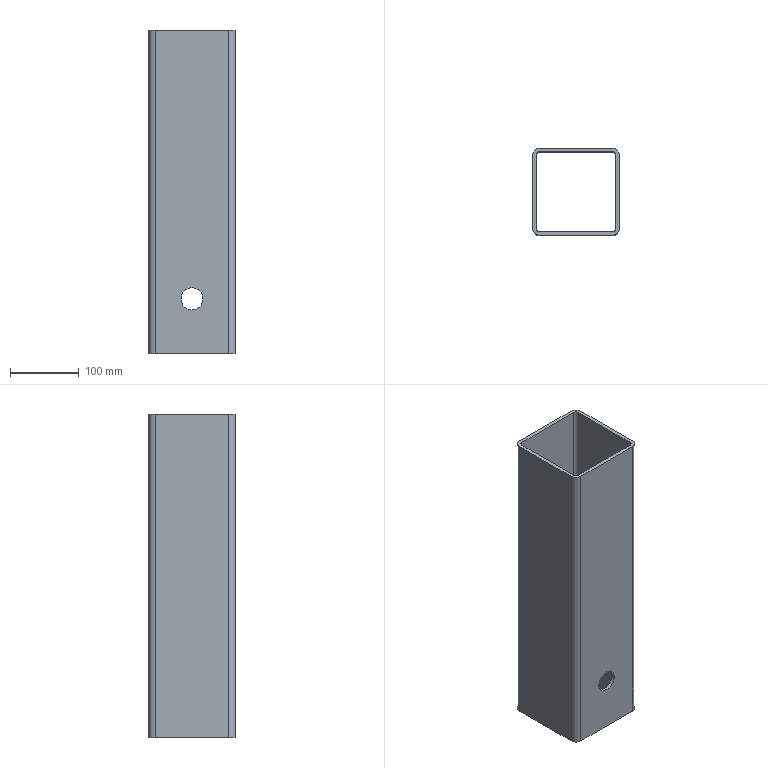Part | SolidWorks | features Attribute 1, Extrusion 1, ICE 1 | 1 solid | 22 faces | box 126 x 126 x 470 mm | volume 1099099 mm3 | cylinder 12 | plane 10 | commonest cylinder face diameters 10 x4 20 x4 32 x4
STEP:
#1=CARTESIAN_POINT('',(0.,-63.,-171.));
#2=VERTEX_POINT('',#1);
#3=CARTESIAN_POINT('',(0.,-63.,-139.));
#4=VERTEX_POINT('',#3);
#5=CARTESIAN_POINT('',(0.,-63.,-155.));
#6=DIRECTION('',(0.,1.,0.));
#7=DIRECTION('',(0.,0.,1.));
#8=AXIS2_PLACEMENT_3D('',#5,#6,#7);
#9=CIRCLE('',#8,16.);
#10=EDGE_CURVE('',#2,#4,#9,.T.);
#11=ORIENTED_EDGE('',*,*,#10,.F.);
#12=CARTESIAN_POINT('',(0.,-58.,-171.));
#13=VERTEX_POINT('',#12);
#14=CARTESIAN_POINT('',(0.,-63.,-171.));
#15=DIRECTION('',(0.,1.,0.));
#16=VECTOR('',#15,1000.);
#17=LINE('',#14,#16);
#18=EDGE_CURVE('',#2,#13,#17,.T.);
#19=ORIENTED_EDGE('',*,*,#18,.T.);
#20=CARTESIAN_POINT('',(0.,-58.,-139.));
#21=VERTEX_POINT('',#20);
#22=CARTESIAN_POINT('',(0.,-58.,-155.));
#23=DIRECTION('',(0.,1.,0.));
#24=DIRECTION('',(0.,0.,1.));
#25=AXIS2_PLACEMENT_3D('',#22,#23,#24);
#26=CIRCLE('',#25,16.);
#27=EDGE_CURVE('',#13,#21,#26,.T.);
#28=ORIENTED_EDGE('',*,*,#27,.T.);
#29=CARTESIAN_POINT('',(0.,-63.,-139.));
#30=DIRECTION('',(0.,1.,0.));
#31=VECTOR('',#30,1000.);
#32=LINE('',#29,#31);
#33=EDGE_CURVE('',#4,#21,#32,.T.);
#34=ORIENTED_EDGE('',*,*,#33,.F.);
#35=EDGE_LOOP('',(#11,#19,#28,#34));
#36=FACE_OUTER_BOUND('',#35,.T.);
#37=CARTESIAN_POINT('',(0.,-63.,-155.));
#38=DIRECTION('',(0.,1.,0.));
#39=DIRECTION('',(0.,0.,1.));
#40=AXIS2_PLACEMENT_3D('',#37,#38,#39);
#41=CYLINDRICAL_SURFACE('',#40,16.);
#42=ADVANCED_FACE('',(#36),#41,.F.);
#43=CARTESIAN_POINT('',(0.,58.,-139.));
#44=VERTEX_POINT('',#43);
#45=CARTESIAN_POINT('',(0.,58.,-171.));
#46=VERTEX_POINT('',#45);
#47=CARTESIAN_POINT('',(0.,58.,-155.));
#48=DIRECTION('',(0.,-1.,0.));
#49=DIRECTION('',(0.,0.,-1.));
#50=AXIS2_PLACEMENT_3D('',#47,#48,#49);
#51=CIRCLE('',#50,16.);
#52=EDGE_CURVE('',#44,#46,#51,.T.);
#53=ORIENTED_EDGE('',*,*,#52,.T.);
#54=CARTESIAN_POINT('',(0.,63.,-171.));
#55=VERTEX_POINT('',#54);
#56=CARTESIAN_POINT('',(0.,-63.,-171.));
#57=DIRECTION('',(0.,1.,0.));
#58=VECTOR('',#57,1000.);
#59=LINE('',#56,#58);
#60=EDGE_CURVE('',#46,#55,#59,.T.);
#61=ORIENTED_EDGE('',*,*,#60,.T.);
#62=CARTESIAN_POINT('',(0.,63.,-139.));
#63=VERTEX_POINT('',#62);
#64=CARTESIAN_POINT('',(0.,63.,-155.));
#65=DIRECTION('',(0.,1.,0.));
#66=DIRECTION('',(0.,0.,1.));
#67=AXIS2_PLACEMENT_3D('',#64,#65,#66);
#68=CIRCLE('',#67,16.);
#69=EDGE_CURVE('',#55,#63,#68,.T.);
#70=ORIENTED_EDGE('',*,*,#69,.T.);
#71=CARTESIAN_POINT('',(0.,-63.,-139.));
#72=DIRECTION('',(0.,1.,0.));
#73=VECTOR('',#72,1000.);
#74=LINE('',#71,#73);
#75=EDGE_CURVE('',#44,#63,#74,.T.);
#76=ORIENTED_EDGE('',*,*,#75,.F.);
#77=EDGE_LOOP('',(#53,#61,#70,#76));
#78=FACE_OUTER_BOUND('',#77,.T.);
#79=CARTESIAN_POINT('',(0.,-63.,-155.));
#80=DIRECTION('',(0.,1.,0.));
#81=DIRECTION('',(0.,0.,1.));
#82=AXIS2_PLACEMENT_3D('',#79,#80,#81);
#83=CYLINDRICAL_SURFACE('',#82,16.);
#84=ADVANCED_FACE('',(#78),#83,.F.);
#85=CARTESIAN_POINT('',(63.,53.,235.));
#86=VERTEX_POINT('',#85);
#87=CARTESIAN_POINT('',(53.,63.,235.));
#88=VERTEX_POINT('',#87);
#89=CARTESIAN_POINT('',(53.,53.,235.));
#90=DIRECTION('',(0.,0.,1.));
#91=DIRECTION('',(1.,0.,0.));
#92=AXIS2_PLACEMENT_3D('',#89,#90,#91);
#93=CIRCLE('',#92,10.);
#94=EDGE_CURVE('',#86,#88,#93,.T.);
#95=ORIENTED_EDGE('',*,*,#94,.T.);
#96=CARTESIAN_POINT('',(-53.,63.,235.));
#97=VERTEX_POINT('',#96);
#98=CARTESIAN_POINT('',(53.,63.,235.));
#99=DIRECTION('',(-1.,0.,0.));
#100=VECTOR('',#99,1000.);
#101=LINE('',#98,#100);
#102=EDGE_CURVE('',#88,#97,#101,.T.);
#103=ORIENTED_EDGE('',*,*,#102,.T.);
#104=CARTESIAN_POINT('',(-63.,53.,235.));
#105=VERTEX_POINT('',#104);
#106=CARTESIAN_POINT('',(-53.,53.,235.));
#107=DIRECTION('',(0.,0.,1.));
#108=DIRECTION('',(1.,0.,0.));
#109=AXIS2_PLACEMENT_3D('',#106,#107,#108);
#110=CIRCLE('',#109,10.);
#111=EDGE_CURVE('',#97,#105,#110,.T.);
#112=ORIENTED_EDGE('',*,*,#111,.T.);
#113=CARTESIAN_POINT('',(-63.,-53.,235.));
#114=VERTEX_POINT('',#113);
#115=CARTESIAN_POINT('',(-63.,-53.,235.));
#116=DIRECTION('',(0.,-1.,0.));
#117=VECTOR('',#116,1000.);
#118=LINE('',#115,#117);
#119=EDGE_CURVE('',#105,#114,#118,.T.);
#120=ORIENTED_EDGE('',*,*,#119,.T.);
#121=CARTESIAN_POINT('',(-53.,-63.,235.));
#122=VERTEX_POINT('',#121);
#123=CARTESIAN_POINT('',(-53.,-53.,235.));
#124=DIRECTION('',(0.,0.,1.));
#125=DIRECTION('',(1.,0.,0.));
#126=AXIS2_PLACEMENT_3D('',#123,#124,#125);
#127=CIRCLE('',#126,10.);
#128=EDGE_CURVE('',#114,#122,#127,.T.);
#129=ORIENTED_EDGE('',*,*,#128,.T.);
#130=CARTESIAN_POINT('',(53.,-63.,235.));
#131=VERTEX_POINT('',#130);
#132=CARTESIAN_POINT('',(-53.,-63.,235.));
#133=DIRECTION('',(1.,0.,0.));
#134=VECTOR('',#133,1000.);
#135=LINE('',#132,#134);
#136=EDGE_CURVE('',#122,#131,#135,.T.);
#137=ORIENTED_EDGE('',*,*,#136,.T.);
#138=CARTESIAN_POINT('',(63.,-53.,235.));
#139=VERTEX_POINT('',#138);
#140=CARTESIAN_POINT('',(53.,-53.,235.));
#141=DIRECTION('',(0.,0.,1.));
#142=DIRECTION('',(1.,0.,0.));
#143=AXIS2_PLACEMENT_3D('',#140,#141,#142);
#144=CIRCLE('',#143,10.);
#145=EDGE_CURVE('',#131,#139,#144,.T.);
#146=ORIENTED_EDGE('',*,*,#145,.T.);
#147=CARTESIAN_POINT('',(63.,53.,235.));
#148=DIRECTION('',(0.,1.,0.));
#149=VECTOR('',#148,1000.);
#150=LINE('',#147,#149);
#151=EDGE_CURVE('',#139,#86,#150,.T.);
#152=ORIENTED_EDGE('',*,*,#151,.T.);
#153=EDGE_LOOP('',(#95,#103,#112,#120,#129,#137,#146,#152));
#154=FACE_OUTER_BOUND('',#153,.T.);
#155=CARTESIAN_POINT('',(-58.,53.,235.));
#156=VERTEX_POINT('',#155);
#157=CARTESIAN_POINT('',(-58.,-53.,235.));
#158=VERTEX_POINT('',#157);
#159=CARTESIAN_POINT('',(-58.,-53.,235.));
#160=DIRECTION('',(0.,-1.,0.));
#161=VECTOR('',#160,1000.);
#162=LINE('',#159,#161);
#163=EDGE_CURVE('',#156,#158,#162,.T.);
#164=ORIENTED_EDGE('',*,*,#163,.F.);
#165=CARTESIAN_POINT('',(-53.,58.,235.));
#166=VERTEX_POINT('',#165);
#167=CARTESIAN_POINT('',(-53.,53.,235.));
#168=DIRECTION('',(0.,0.,1.));
#169=DIRECTION('',(1.,0.,0.));
#170=AXIS2_PLACEMENT_3D('',#167,#168,#169);
#171=CIRCLE('',#170,5.);
#172=EDGE_CURVE('',#166,#156,#171,.T.);
#173=ORIENTED_EDGE('',*,*,#172,.F.);
#174=CARTESIAN_POINT('',(53.,58.,235.));
#175=VERTEX_POINT('',#174);
#176=CARTESIAN_POINT('',(53.,58.,235.));
#177=DIRECTION('',(-1.,0.,0.));
#178=VECTOR('',#177,1000.);
#179=LINE('',#176,#178);
#180=EDGE_CURVE('',#175,#166,#179,.T.);
#181=ORIENTED_EDGE('',*,*,#180,.F.);
#182=CARTESIAN_POINT('',(58.,53.,235.));
#183=VERTEX_POINT('',#182);
#184=CARTESIAN_POINT('',(53.,53.,235.));
#185=DIRECTION('',(0.,0.,1.));
#186=DIRECTION('',(1.,0.,0.));
#187=AXIS2_PLACEMENT_3D('',#184,#185,#186);
#188=CIRCLE('',#187,5.);
#189=EDGE_CURVE('',#183,#175,#188,.T.);
#190=ORIENTED_EDGE('',*,*,#189,.F.);
#191=CARTESIAN_POINT('',(58.,-53.,235.));
#192=VERTEX_POINT('',#191);
#193=CARTESIAN_POINT('',(58.,53.,235.));
#194=DIRECTION('',(0.,1.,0.));
#195=VECTOR('',#194,1000.);
#196=LINE('',#193,#195);
#197=EDGE_CURVE('',#192,#183,#196,.T.);
#198=ORIENTED_EDGE('',*,*,#197,.F.);
#199=CARTESIAN_POINT('',(53.,-58.,235.));
#200=VERTEX_POINT('',#199);
#201=CARTESIAN_POINT('',(53.,-53.,235.));
#202=DIRECTION('',(0.,0.,1.));
#203=DIRECTION('',(1.,0.,0.));
#204=AXIS2_PLACEMENT_3D('',#201,#202,#203);
#205=CIRCLE('',#204,5.);
#206=EDGE_CURVE('',#200,#192,#205,.T.);
#207=ORIENTED_EDGE('',*,*,#206,.F.);
#208=CARTESIAN_POINT('',(-53.,-58.,235.));
#209=VERTEX_POINT('',#208);
#210=CARTESIAN_POINT('',(-53.,-58.,235.));
#211=DIRECTION('',(1.,0.,0.));
#212=VECTOR('',#211,1000.);
#213=LINE('',#210,#212);
#214=EDGE_CURVE('',#209,#200,#213,.T.);
#215=ORIENTED_EDGE('',*,*,#214,.F.);
#216=CARTESIAN_POINT('',(-53.,-53.,235.));
#217=DIRECTION('',(0.,0.,1.));
#218=DIRECTION('',(1.,0.,0.));
#219=AXIS2_PLACEMENT_3D('',#216,#217,#218);
#220=CIRCLE('',#219,5.);
#221=EDGE_CURVE('',#158,#209,#220,.T.);
#222=ORIENTED_EDGE('',*,*,#221,.F.);
#223=EDGE_LOOP('',(#164,#173,#181,#190,#198,#207,#215,#222));
#224=FACE_BOUND('',#223,.T.);
#225=CARTESIAN_POINT('',(53.,53.,235.));
#226=DIRECTION('',(0.,0.,1.));
#227=DIRECTION('',(1.,0.,0.));
#228=AXIS2_PLACEMENT_3D('',#225,#226,#227);
#229=PLANE('',#228);
#230=ADVANCED_FACE('',(#154,#224),#229,.T.);
#231=CARTESIAN_POINT('',(63.,53.,-235.));
#232=VERTEX_POINT('',#231);
#233=CARTESIAN_POINT('',(53.,63.,-235.));
#234=VERTEX_POINT('',#233);
#235=CARTESIAN_POINT('',(53.,53.,-235.));
#236=DIRECTION('',(0.,0.,1.));
#237=DIRECTION('',(1.,0.,0.));
#238=AXIS2_PLACEMENT_3D('',#235,#236,#237);
#239=CIRCLE('',#238,10.);
#240=EDGE_CURVE('',#232,#234,#239,.T.);
#241=ORIENTED_EDGE('',*,*,#240,.F.);
#242=CARTESIAN_POINT('',(63.,-53.,-235.));
#243=VERTEX_POINT('',#242);
#244=CARTESIAN_POINT('',(63.,53.,-235.));
#245=DIRECTION('',(0.,1.,0.));
#246=VECTOR('',#245,1000.);
#247=LINE('',#244,#246);
#248=EDGE_CURVE('',#243,#232,#247,.T.);
#249=ORIENTED_EDGE('',*,*,#248,.F.);
#250=CARTESIAN_POINT('',(53.,-63.,-235.));
#251=VERTEX_POINT('',#250);
#252=CARTESIAN_POINT('',(53.,-53.,-235.));
#253=DIRECTION('',(0.,0.,1.));
#254=DIRECTION('',(1.,0.,0.));
#255=AXIS2_PLACEMENT_3D('',#252,#253,#254);
#256=CIRCLE('',#255,10.);
#257=EDGE_CURVE('',#251,#243,#256,.T.);
#258=ORIENTED_EDGE('',*,*,#257,.F.);
#259=CARTESIAN_POINT('',(-53.,-63.,-235.));
#260=VERTEX_POINT('',#259);
#261=CARTESIAN_POINT('',(-53.,-63.,-235.));
#262=DIRECTION('',(1.,0.,0.));
#263=VECTOR('',#262,1000.);
#264=LINE('',#261,#263);
#265=EDGE_CURVE('',#260,#251,#264,.T.);
#266=ORIENTED_EDGE('',*,*,#265,.F.);
#267=CARTESIAN_POINT('',(-63.,-53.,-235.));
#268=VERTEX_POINT('',#267);
#269=CARTESIAN_POINT('',(-53.,-53.,-235.));
#270=DIRECTION('',(0.,0.,1.));
#271=DIRECTION('',(1.,0.,0.));
#272=AXIS2_PLACEMENT_3D('',#269,#270,#271);
#273=CIRCLE('',#272,10.);
#274=EDGE_CURVE('',#268,#260,#273,.T.);
#275=ORIENTED_EDGE('',*,*,#274,.F.);
#276=CARTESIAN_POINT('',(-63.,53.,-235.));
#277=VERTEX_POINT('',#276);
#278=CARTESIAN_POINT('',(-63.,-53.,-235.));
#279=DIRECTION('',(0.,-1.,0.));
#280=VECTOR('',#279,1000.);
#281=LINE('',#278,#280);
#282=EDGE_CURVE('',#277,#268,#281,.T.);
#283=ORIENTED_EDGE('',*,*,#282,.F.);
#284=CARTESIAN_POINT('',(-53.,63.,-235.));
#285=VERTEX_POINT('',#284);
#286=CARTESIAN_POINT('',(-53.,53.,-235.));
#287=DIRECTION('',(0.,0.,1.));
#288=DIRECTION('',(1.,0.,0.));
#289=AXIS2_PLACEMENT_3D('',#286,#287,#288);
#290=CIRCLE('',#289,10.);
#291=EDGE_CURVE('',#285,#277,#290,.T.);
#292=ORIENTED_EDGE('',*,*,#291,.F.);
#293=CARTESIAN_POINT('',(53.,63.,-235.));
#294=DIRECTION('',(-1.,0.,0.));
#295=VECTOR('',#294,1000.);
#296=LINE('',#293,#295);
#297=EDGE_CURVE('',#234,#285,#296,.T.);
#298=ORIENTED_EDGE('',*,*,#297,.F.);
#299=EDGE_LOOP('',(#241,#249,#258,#266,#275,#283,#292,#298));
#300=FACE_OUTER_BOUND('',#299,.T.);
#301=CARTESIAN_POINT('',(-53.,58.,-235.));
#302=VERTEX_POINT('',#301);
#303=CARTESIAN_POINT('',(-58.,53.,-235.));
#304=VERTEX_POINT('',#303);
#305=CARTESIAN_POINT('',(-53.,53.,-235.));
#306=DIRECTION('',(0.,0.,1.));
#307=DIRECTION('',(1.,0.,0.));
#308=AXIS2_PLACEMENT_3D('',#305,#306,#307);
#309=CIRCLE('',#308,5.);
#310=EDGE_CURVE('',#302,#304,#309,.T.);
#311=ORIENTED_EDGE('',*,*,#310,.T.);
#312=CARTESIAN_POINT('',(-58.,-53.,-235.));
#313=VERTEX_POINT('',#312);
#314=CARTESIAN_POINT('',(-58.,-53.,-235.));
#315=DIRECTION('',(0.,-1.,0.));
#316=VECTOR('',#315,1000.);
#317=LINE('',#314,#316);
#318=EDGE_CURVE('',#304,#313,#317,.T.);
#319=ORIENTED_EDGE('',*,*,#318,.T.);
#320=CARTESIAN_POINT('',(-53.,-58.,-235.));
#321=VERTEX_POINT('',#320);
#322=CARTESIAN_POINT('',(-53.,-53.,-235.));
#323=DIRECTION('',(0.,0.,1.));
#324=DIRECTION('',(1.,0.,0.));
#325=AXIS2_PLACEMENT_3D('',#322,#323,#324);
#326=CIRCLE('',#325,5.);
#327=EDGE_CURVE('',#313,#321,#326,.T.);
#328=ORIENTED_EDGE('',*,*,#327,.T.);
#329=CARTESIAN_POINT('',(53.,-58.,-235.));
#330=VERTEX_POINT('',#329);
#331=CARTESIAN_POINT('',(-53.,-58.,-235.));
#332=DIRECTION('',(1.,0.,0.));
#333=VECTOR('',#332,1000.);
#334=LINE('',#331,#333);
#335=EDGE_CURVE('',#321,#330,#334,.T.);
#336=ORIENTED_EDGE('',*,*,#335,.T.);
#337=CARTESIAN_POINT('',(58.,-53.,-235.));
#338=VERTEX_POINT('',#337);
#339=CARTESIAN_POINT('',(53.,-53.,-235.));
#340=DIRECTION('',(0.,0.,1.));
#341=DIRECTION('',(1.,0.,0.));
#342=AXIS2_PLACEMENT_3D('',#339,#340,#341);
#343=CIRCLE('',#342,5.);
#344=EDGE_CURVE('',#330,#338,#343,.T.);
#345=ORIENTED_EDGE('',*,*,#344,.T.);
#346=CARTESIAN_POINT('',(58.,53.,-235.));
#347=VERTEX_POINT('',#346);
#348=CARTESIAN_POINT('',(58.,53.,-235.));
#349=DIRECTION('',(0.,1.,0.));
#350=VECTOR('',#349,1000.);
#351=LINE('',#348,#350);
#352=EDGE_CURVE('',#338,#347,#351,.T.);
#353=ORIENTED_EDGE('',*,*,#352,.T.);
#354=CARTESIAN_POINT('',(53.,58.,-235.));
#355=VERTEX_POINT('',#354);
#356=CARTESIAN_POINT('',(53.,53.,-235.));
#357=DIRECTION('',(0.,0.,1.));
#358=DIRECTION('',(1.,0.,0.));
#359=AXIS2_PLACEMENT_3D('',#356,#357,#358);
#360=CIRCLE('',#359,5.);
#361=EDGE_CURVE('',#347,#355,#360,.T.);
#362=ORIENTED_EDGE('',*,*,#361,.T.);
#363=CARTESIAN_POINT('',(53.,58.,-235.));
#364=DIRECTION('',(-1.,0.,0.));
#365=VECTOR('',#364,1000.);
#366=LINE('',#363,#365);
#367=EDGE_CURVE('',#355,#302,#366,.T.);
#368=ORIENTED_EDGE('',*,*,#367,.T.);
#369=EDGE_LOOP('',(#311,#319,#328,#336,#345,#353,#362,#368));
#370=FACE_BOUND('',#369,.T.);
#371=CARTESIAN_POINT('',(53.,53.,-235.));
#372=DIRECTION('',(0.,0.,1.));
#373=DIRECTION('',(1.,0.,0.));
#374=AXIS2_PLACEMENT_3D('',#371,#372,#373);
#375=PLANE('',#374);
#376=ADVANCED_FACE('',(#300,#370),#375,.F.);
#377=ORIENTED_EDGE('',*,*,#240,.T.);
#378=CARTESIAN_POINT('',(53.,63.,235.));
#379=DIRECTION('',(0.,0.,-1.));
#380=VECTOR('',#379,1000.);
#381=LINE('',#378,#380);
#382=EDGE_CURVE('',#88,#234,#381,.T.);
#383=ORIENTED_EDGE('',*,*,#382,.F.);
#384=ORIENTED_EDGE('',*,*,#94,.F.);
#385=CARTESIAN_POINT('',(63.,53.,235.));
#386=DIRECTION('',(0.,0.,-1.));
#387=VECTOR('',#386,1000.);
#388=LINE('',#385,#387);
#389=EDGE_CURVE('',#86,#232,#388,.T.);
#390=ORIENTED_EDGE('',*,*,#389,.T.);
#391=EDGE_LOOP('',(#377,#383,#384,#390));
#392=FACE_OUTER_BOUND('',#391,.T.);
#393=CARTESIAN_POINT('',(53.,53.,235.));
#394=DIRECTION('',(0.,0.,-1.));
#395=DIRECTION('',(-1.,0.,0.));
#396=AXIS2_PLACEMENT_3D('',#393,#394,#395);
#397=CYLINDRICAL_SURFACE('',#396,10.);
#398=ADVANCED_FACE('',(#392),#397,.T.);
#399=CARTESIAN_POINT('',(0.,63.,-155.));
#400=DIRECTION('',(0.,1.,0.));
#401=DIRECTION('',(0.,0.,1.));
#402=AXIS2_PLACEMENT_3D('',#399,#400,#401);
#403=CIRCLE('',#402,16.);
#404=EDGE_CURVE('',#63,#55,#403,.T.);
#405=ORIENTED_EDGE('',*,*,#404,.F.);
#406=ORIENTED_EDGE('',*,*,#69,.F.);
#407=EDGE_LOOP('',(#405,#406));
#408=FACE_BOUND('',#407,.T.);
#409=ORIENTED_EDGE('',*,*,#297,.T.);
#410=CARTESIAN_POINT('',(-53.,63.,235.));
#411=DIRECTION('',(0.,0.,-1.));
#412=VECTOR('',#411,1000.);
#413=LINE('',#410,#412);
#414=EDGE_CURVE('',#97,#285,#413,.T.);
#415=ORIENTED_EDGE('',*,*,#414,.F.);
#416=ORIENTED_EDGE('',*,*,#102,.F.);
#417=ORIENTED_EDGE('',*,*,#382,.T.);
#418=EDGE_LOOP('',(#409,#415,#416,#417));
#419=FACE_OUTER_BOUND('',#418,.T.);
#420=CARTESIAN_POINT('',(53.,63.,235.));
#421=DIRECTION('',(0.,-1.,0.));
#422=DIRECTION('',(0.,0.,-1.));
#423=AXIS2_PLACEMENT_3D('',#420,#421,#422);
#424=PLANE('',#423);
#425=ADVANCED_FACE('',(#408,#419),#424,.F.);
#426=ORIENTED_EDGE('',*,*,#291,.T.);
#427=CARTESIAN_POINT('',(-63.,53.,235.));
#428=DIRECTION('',(0.,0.,-1.));
#429=VECTOR('',#428,1000.);
#430=LINE('',#427,#429);
#431=EDGE_CURVE('',#105,#277,#430,.T.);
#432=ORIENTED_EDGE('',*,*,#431,.F.);
#433=ORIENTED_EDGE('',*,*,#111,.F.);
#434=ORIENTED_EDGE('',*,*,#414,.T.);
#435=EDGE_LOOP('',(#426,#432,#433,#434));
#436=FACE_OUTER_BOUND('',#435,.T.);
#437=CARTESIAN_POINT('',(-53.,53.,235.));
#438=DIRECTION('',(0.,0.,-1.));
#439=DIRECTION('',(-1.,0.,0.));
#440=AXIS2_PLACEMENT_3D('',#437,#438,#439);
#441=CYLINDRICAL_SURFACE('',#440,10.);
#442=ADVANCED_FACE('',(#436),#441,.T.);
#443=ORIENTED_EDGE('',*,*,#282,.T.);
#444=CARTESIAN_POINT('',(-63.,-53.,235.));
#445=DIRECTION('',(0.,0.,-1.));
#446=VECTOR('',#445,1000.);
#447=LINE('',#444,#446);
#448=EDGE_CURVE('',#114,#268,#447,.T.);
#449=ORIENTED_EDGE('',*,*,#448,.F.);
#450=ORIENTED_EDGE('',*,*,#119,.F.);
#451=ORIENTED_EDGE('',*,*,#431,.T.);
#452=EDGE_LOOP('',(#443,#449,#450,#451));
#453=FACE_OUTER_BOUND('',#452,.T.);
#454=CARTESIAN_POINT('',(-63.,-53.,235.));
#455=DIRECTION('',(1.,0.,0.));
#456=DIRECTION('',(0.,0.,-1.));
#457=AXIS2_PLACEMENT_3D('',#454,#455,#456);
#458=PLANE('',#457);
#459=ADVANCED_FACE('',(#453),#458,.F.);
#460=ORIENTED_EDGE('',*,*,#274,.T.);
#461=CARTESIAN_POINT('',(-53.,-63.,235.));
#462=DIRECTION('',(0.,0.,-1.));
#463=VECTOR('',#462,1000.);
#464=LINE('',#461,#463);
#465=EDGE_CURVE('',#122,#260,#464,.T.);
#466=ORIENTED_EDGE('',*,*,#465,.F.);
#467=ORIENTED_EDGE('',*,*,#128,.F.);
#468=ORIENTED_EDGE('',*,*,#448,.T.);
#469=EDGE_LOOP('',(#460,#466,#467,#468));
#470=FACE_OUTER_BOUND('',#469,.T.);
#471=CARTESIAN_POINT('',(-53.,-53.,235.));
#472=DIRECTION('',(0.,0.,-1.));
#473=DIRECTION('',(-1.,0.,0.));
#474=AXIS2_PLACEMENT_3D('',#471,#472,#473);
#475=CYLINDRICAL_SURFACE('',#474,10.);
#476=ADVANCED_FACE('',(#470),#475,.T.);
#477=CARTESIAN_POINT('',(0.,-63.,-155.));
#478=DIRECTION('',(0.,1.,0.));
#479=DIRECTION('',(0.,0.,1.));
#480=AXIS2_PLACEMENT_3D('',#477,#478,#479);
#481=CIRCLE('',#480,16.);
#482=EDGE_CURVE('',#4,#2,#481,.T.);
#483=ORIENTED_EDGE('',*,*,#482,.T.);
#484=ORIENTED_EDGE('',*,*,#10,.T.);
#485=EDGE_LOOP('',(#483,#484));
#486=FACE_BOUND('',#485,.T.);
#487=ORIENTED_EDGE('',*,*,#265,.T.);
#488=CARTESIAN_POINT('',(53.,-63.,235.));
#489=DIRECTION('',(0.,0.,-1.));
#490=VECTOR('',#489,1000.);
#491=LINE('',#488,#490);
#492=EDGE_CURVE('',#131,#251,#491,.T.);
#493=ORIENTED_EDGE('',*,*,#492,.F.);
#494=ORIENTED_EDGE('',*,*,#136,.F.);
#495=ORIENTED_EDGE('',*,*,#465,.T.);
#496=EDGE_LOOP('',(#487,#493,#494,#495));
#497=FACE_OUTER_BOUND('',#496,.T.);
#498=CARTESIAN_POINT('',(-53.,-63.,235.));
#499=DIRECTION('',(0.,1.,0.));
#500=DIRECTION('',(0.,0.,1.));
#501=AXIS2_PLACEMENT_3D('',#498,#499,#500);
#502=PLANE('',#501);
#503=ADVANCED_FACE('',(#486,#497),#502,.F.);
#504=ORIENTED_EDGE('',*,*,#257,.T.);
#505=CARTESIAN_POINT('',(63.,-53.,235.));
#506=DIRECTION('',(0.,0.,-1.));
#507=VECTOR('',#506,1000.);
#508=LINE('',#505,#507);
#509=EDGE_CURVE('',#139,#243,#508,.T.);
#510=ORIENTED_EDGE('',*,*,#509,.F.);
#511=ORIENTED_EDGE('',*,*,#145,.F.);
#512=ORIENTED_EDGE('',*,*,#492,.T.);
#513=EDGE_LOOP('',(#504,#510,#511,#512));
#514=FACE_OUTER_BOUND('',#513,.T.);
#515=CARTESIAN_POINT('',(53.,-53.,235.));
#516=DIRECTION('',(0.,0.,-1.));
#517=DIRECTION('',(-1.,0.,0.));
#518=AXIS2_PLACEMENT_3D('',#515,#516,#517);
#519=CYLINDRICAL_SURFACE('',#518,10.);
#520=ADVANCED_FACE('',(#514),#519,.T.);
#521=ORIENTED_EDGE('',*,*,#248,.T.);
#522=ORIENTED_EDGE('',*,*,#389,.F.);
#523=ORIENTED_EDGE('',*,*,#151,.F.);
#524=ORIENTED_EDGE('',*,*,#509,.T.);
#525=EDGE_LOOP('',(#521,#522,#523,#524));
#526=FACE_OUTER_BOUND('',#525,.T.);
#527=CARTESIAN_POINT('',(63.,53.,235.));
#528=DIRECTION('',(-1.,0.,0.));
#529=DIRECTION('',(0.,0.,1.));
#530=AXIS2_PLACEMENT_3D('',#527,#528,#529);
#531=PLANE('',#530);
#532=ADVANCED_FACE('',(#526),#531,.F.);
#533=ORIENTED_EDGE('',*,*,#310,.F.);
#534=CARTESIAN_POINT('',(-53.,58.,235.));
#535=DIRECTION('',(0.,0.,-1.));
#536=VECTOR('',#535,1000.);
#537=LINE('',#534,#536);
#538=EDGE_CURVE('',#166,#302,#537,.T.);
#539=ORIENTED_EDGE('',*,*,#538,.F.);
#540=ORIENTED_EDGE('',*,*,#172,.T.);
#541=CARTESIAN_POINT('',(-58.,53.,235.));
#542=DIRECTION('',(0.,0.,-1.));
#543=VECTOR('',#542,1000.);
#544=LINE('',#541,#543);
#545=EDGE_CURVE('',#156,#304,#544,.T.);
#546=ORIENTED_EDGE('',*,*,#545,.T.);
#547=EDGE_LOOP('',(#533,#539,#540,#546));
#548=FACE_OUTER_BOUND('',#547,.T.);
#549=CARTESIAN_POINT('',(-53.,53.,235.));
#550=DIRECTION('',(0.,0.,-1.));
#551=DIRECTION('',(-1.,0.,0.));
#552=AXIS2_PLACEMENT_3D('',#549,#550,#551);
#553=CYLINDRICAL_SURFACE('',#552,5.);
#554=ADVANCED_FACE('',(#548),#553,.F.);
#555=ORIENTED_EDGE('',*,*,#318,.F.);
#556=ORIENTED_EDGE('',*,*,#545,.F.);
#557=ORIENTED_EDGE('',*,*,#163,.T.);
#558=CARTESIAN_POINT('',(-58.,-53.,235.));
#559=DIRECTION('',(0.,0.,-1.));
#560=VECTOR('',#559,1000.);
#561=LINE('',#558,#560);
#562=EDGE_CURVE('',#158,#313,#561,.T.);
#563=ORIENTED_EDGE('',*,*,#562,.T.);
#564=EDGE_LOOP('',(#555,#556,#557,#563));
#565=FACE_OUTER_BOUND('',#564,.T.);
#566=CARTESIAN_POINT('',(-58.,-53.,235.));
#567=DIRECTION('',(1.,0.,0.));
#568=DIRECTION('',(0.,0.,-1.));
#569=AXIS2_PLACEMENT_3D('',#566,#567,#568);
#570=PLANE('',#569);
#571=ADVANCED_FACE('',(#565),#570,.T.);
#572=ORIENTED_EDGE('',*,*,#327,.F.);
#573=ORIENTED_EDGE('',*,*,#562,.F.);
#574=ORIENTED_EDGE('',*,*,#221,.T.);
#575=CARTESIAN_POINT('',(-53.,-58.,235.));
#576=DIRECTION('',(0.,0.,-1.));
#577=VECTOR('',#576,1000.);
#578=LINE('',#575,#577);
#579=EDGE_CURVE('',#209,#321,#578,.T.);
#580=ORIENTED_EDGE('',*,*,#579,.T.);
#581=EDGE_LOOP('',(#572,#573,#574,#580));
#582=FACE_OUTER_BOUND('',#581,.T.);
#583=CARTESIAN_POINT('',(-53.,-53.,235.));
#584=DIRECTION('',(0.,0.,-1.));
#585=DIRECTION('',(-1.,0.,0.));
#586=AXIS2_PLACEMENT_3D('',#583,#584,#585);
#587=CYLINDRICAL_SURFACE('',#586,5.);
#588=ADVANCED_FACE('',(#582),#587,.F.);
#589=CARTESIAN_POINT('',(0.,-58.,-155.));
#590=DIRECTION('',(0.,1.,0.));
#591=DIRECTION('',(0.,0.,1.));
#592=AXIS2_PLACEMENT_3D('',#589,#590,#591);
#593=CIRCLE('',#592,16.);
#594=EDGE_CURVE('',#21,#13,#593,.T.);
#595=ORIENTED_EDGE('',*,*,#594,.F.);
#596=ORIENTED_EDGE('',*,*,#27,.F.);
#597=EDGE_LOOP('',(#595,#596));
#598=FACE_BOUND('',#597,.T.);
#599=ORIENTED_EDGE('',*,*,#335,.F.);
#600=ORIENTED_EDGE('',*,*,#579,.F.);
#601=ORIENTED_EDGE('',*,*,#214,.T.);
#602=CARTESIAN_POINT('',(53.,-58.,235.));
#603=DIRECTION('',(0.,0.,-1.));
#604=VECTOR('',#603,1000.);
#605=LINE('',#602,#604);
#606=EDGE_CURVE('',#200,#330,#605,.T.);
#607=ORIENTED_EDGE('',*,*,#606,.T.);
#608=EDGE_LOOP('',(#599,#600,#601,#607));
#609=FACE_OUTER_BOUND('',#608,.T.);
#610=CARTESIAN_POINT('',(-53.,-58.,235.));
#611=DIRECTION('',(0.,1.,0.));
#612=DIRECTION('',(0.,0.,1.));
#613=AXIS2_PLACEMENT_3D('',#610,#611,#612);
#614=PLANE('',#613);
#615=ADVANCED_FACE('',(#598,#609),#614,.T.);
#616=ORIENTED_EDGE('',*,*,#344,.F.);
#617=ORIENTED_EDGE('',*,*,#606,.F.);
#618=ORIENTED_EDGE('',*,*,#206,.T.);
#619=CARTESIAN_POINT('',(58.,-53.,235.));
#620=DIRECTION('',(0.,0.,-1.));
#621=VECTOR('',#620,1000.);
#622=LINE('',#619,#621);
#623=EDGE_CURVE('',#192,#338,#622,.T.);
#624=ORIENTED_EDGE('',*,*,#623,.T.);
#625=EDGE_LOOP('',(#616,#617,#618,#624));
#626=FACE_OUTER_BOUND('',#625,.T.);
#627=CARTESIAN_POINT('',(53.,-53.,235.));
#628=DIRECTION('',(0.,0.,-1.));
#629=DIRECTION('',(-1.,0.,0.));
#630=AXIS2_PLACEMENT_3D('',#627,#628,#629);
#631=CYLINDRICAL_SURFACE('',#630,5.);
#632=ADVANCED_FACE('',(#626),#631,.F.);
#633=ORIENTED_EDGE('',*,*,#352,.F.);
#634=ORIENTED_EDGE('',*,*,#623,.F.);
#635=ORIENTED_EDGE('',*,*,#197,.T.);
#636=CARTESIAN_POINT('',(58.,53.,235.));
#637=DIRECTION('',(0.,0.,-1.));
#638=VECTOR('',#637,1000.);
#639=LINE('',#636,#638);
#640=EDGE_CURVE('',#183,#347,#639,.T.);
#641=ORIENTED_EDGE('',*,*,#640,.T.);
#642=EDGE_LOOP('',(#633,#634,#635,#641));
#643=FACE_OUTER_BOUND('',#642,.T.);
#644=CARTESIAN_POINT('',(58.,53.,235.));
#645=DIRECTION('',(-1.,0.,0.));
#646=DIRECTION('',(0.,0.,1.));
#647=AXIS2_PLACEMENT_3D('',#644,#645,#646);
#648=PLANE('',#647);
#649=ADVANCED_FACE('',(#643),#648,.T.);
#650=ORIENTED_EDGE('',*,*,#361,.F.);
#651=ORIENTED_EDGE('',*,*,#640,.F.);
#652=ORIENTED_EDGE('',*,*,#189,.T.);
#653=CARTESIAN_POINT('',(53.,58.,235.));
#654=DIRECTION('',(0.,0.,-1.));
#655=VECTOR('',#654,1000.);
#656=LINE('',#653,#655);
#657=EDGE_CURVE('',#175,#355,#656,.T.);
#658=ORIENTED_EDGE('',*,*,#657,.T.);
#659=EDGE_LOOP('',(#650,#651,#652,#658));
#660=FACE_OUTER_BOUND('',#659,.T.);
#661=CARTESIAN_POINT('',(53.,53.,235.));
#662=DIRECTION('',(0.,0.,-1.));
#663=DIRECTION('',(-1.,0.,0.));
#664=AXIS2_PLACEMENT_3D('',#661,#662,#663);
#665=CYLINDRICAL_SURFACE('',#664,5.);
#666=ADVANCED_FACE('',(#660),#665,.F.);
#667=ORIENTED_EDGE('',*,*,#52,.F.);
#668=CARTESIAN_POINT('',(0.,58.,-155.));
#669=DIRECTION('',(0.,-1.,0.));
#670=DIRECTION('',(0.,0.,-1.));
#671=AXIS2_PLACEMENT_3D('',#668,#669,#670);
#672=CIRCLE('',#671,16.);
#673=EDGE_CURVE('',#46,#44,#672,.T.);
#674=ORIENTED_EDGE('',*,*,#673,.F.);
#675=EDGE_LOOP('',(#667,#674));
#676=FACE_BOUND('',#675,.T.);
#677=ORIENTED_EDGE('',*,*,#367,.F.);
#678=ORIENTED_EDGE('',*,*,#657,.F.);
#679=ORIENTED_EDGE('',*,*,#180,.T.);
#680=ORIENTED_EDGE('',*,*,#538,.T.);
#681=EDGE_LOOP('',(#677,#678,#679,#680));
#682=FACE_OUTER_BOUND('',#681,.T.);
#683=CARTESIAN_POINT('',(53.,58.,235.));
#684=DIRECTION('',(0.,-1.,0.));
#685=DIRECTION('',(0.,0.,-1.));
#686=AXIS2_PLACEMENT_3D('',#683,#684,#685);
#687=PLANE('',#686);
#688=ADVANCED_FACE('',(#676,#682),#687,.T.);
#689=ORIENTED_EDGE('',*,*,#60,.F.);
#690=ORIENTED_EDGE('',*,*,#673,.T.);
#691=ORIENTED_EDGE('',*,*,#75,.T.);
#692=ORIENTED_EDGE('',*,*,#404,.T.);
#693=EDGE_LOOP('',(#689,#690,#691,#692));
#694=FACE_OUTER_BOUND('',#693,.T.);
#695=CARTESIAN_POINT('',(0.,-63.,-155.));
#696=DIRECTION('',(0.,1.,0.));
#697=DIRECTION('',(0.,0.,1.));
#698=AXIS2_PLACEMENT_3D('',#695,#696,#697);
#699=CYLINDRICAL_SURFACE('',#698,16.);
#700=ADVANCED_FACE('',(#694),#699,.F.);
#701=ORIENTED_EDGE('',*,*,#18,.F.);
#702=ORIENTED_EDGE('',*,*,#482,.F.);
#703=ORIENTED_EDGE('',*,*,#33,.T.);
#704=ORIENTED_EDGE('',*,*,#594,.T.);
#705=EDGE_LOOP('',(#701,#702,#703,#704));
#706=FACE_OUTER_BOUND('',#705,.T.);
#707=CARTESIAN_POINT('',(0.,-63.,-155.));
#708=DIRECTION('',(0.,1.,0.));
#709=DIRECTION('',(0.,0.,1.));
#710=AXIS2_PLACEMENT_3D('',#707,#708,#709);
#711=CYLINDRICAL_SURFACE('',#710,16.);
#712=ADVANCED_FACE('',(#706),#711,.F.);
#713=CLOSED_SHELL('',(#42,#84,#230,#376,#398,#425,#442,#459,#476,#503,#520,#532,#554,#571,#588,#615,#632,#649,#666,#688,#700,#712));
#714=MANIFOLD_SOLID_BREP('',#713);
#715=CARTESIAN_POINT('',(0.,0.,0.));
#716=DIRECTION('',(0.,0.,1.));
#717=DIRECTION('',(1.,0.,0.));
#718=AXIS2_PLACEMENT_3D('',#715,#716,#717);
#719=(LENGTH_UNIT()NAMED_UNIT(*)SI_UNIT(.MILLI.,.METRE.));
#720=UNCERTAINTY_MEASURE_WITH_UNIT(LENGTH_MEASURE(0.00001),#719,'','');
#721=(NAMED_UNIT(*)PLANE_ANGLE_UNIT()SI_UNIT($,.RADIAN.));
#722=(NAMED_UNIT(*)SI_UNIT($,.STERADIAN.)SOLID_ANGLE_UNIT());
#723=(GEOMETRIC_REPRESENTATION_CONTEXT(3)GLOBAL_UNCERTAINTY_ASSIGNED_CONTEXT((#720))GLOBAL_UNIT_ASSIGNED_CONTEXT((#719,#721,#722))REPRESENTATION_CONTEXT('',''));
#724=ADVANCED_BREP_SHAPE_REPRESENTATION('',(#714,#718),#723);